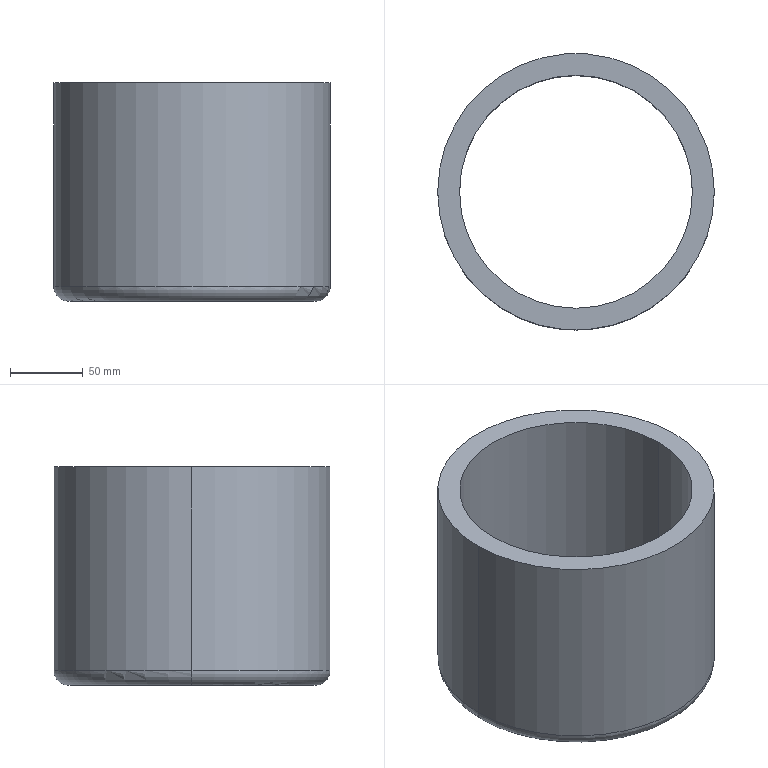Part | SolidWorks | features Extrusion 1, Fillet 1 | 1 solid | 8 faces | box 190 x 190 x 150 mm | volume 1224494 mm3 | cylinder 4 | torus 2 | plane 2 | commonest cylinder face diameters 160 x2 190 x2
STEP:
#1=CARTESIAN_POINT('',(-684.884,-90.,-50.));
#2=VERTEX_POINT('',#1);
#3=CARTESIAN_POINT('',(-514.884,-90.,-50.));
#4=VERTEX_POINT('',#3);
#5=CARTESIAN_POINT('',(-599.884,-90.,-50.));
#6=DIRECTION('',(0.,0.,-1.));
#7=DIRECTION('',(1.,0.,0.));
#8=AXIS2_PLACEMENT_3D('',#5,#6,#7);
#9=CIRCLE('',#8,85.);
#10=EDGE_CURVE('',#2,#4,#9,.T.);
#11=ORIENTED_EDGE('',*,*,#10,.F.);
#12=CARTESIAN_POINT('',(-694.884,-90.,-40.));
#13=VERTEX_POINT('',#12);
#14=CARTESIAN_POINT('',(-684.884,-90.,-40.));
#15=DIRECTION('',(0.,1.,0.));
#16=DIRECTION('',(-1.,0.,0.));
#17=AXIS2_PLACEMENT_3D('',#14,#15,#16);
#18=CIRCLE('',#17,10.);
#19=EDGE_CURVE('',#2,#13,#18,.T.);
#20=ORIENTED_EDGE('',*,*,#19,.T.);
#21=CARTESIAN_POINT('',(-504.884,-90.,-40.));
#22=VERTEX_POINT('',#21);
#23=CARTESIAN_POINT('',(-599.884,-90.,-40.));
#24=DIRECTION('',(0.,0.,1.));
#25=DIRECTION('',(1.,0.,0.));
#26=AXIS2_PLACEMENT_3D('',#23,#24,#25);
#27=CIRCLE('',#26,95.);
#28=EDGE_CURVE('',#22,#13,#27,.T.);
#29=ORIENTED_EDGE('',*,*,#28,.F.);
#30=CARTESIAN_POINT('',(-514.884,-90.,-40.));
#31=DIRECTION('',(0.,-1.,0.));
#32=DIRECTION('',(0.,0.,-1.));
#33=AXIS2_PLACEMENT_3D('',#30,#31,#32);
#34=CIRCLE('',#33,10.);
#35=EDGE_CURVE('',#4,#22,#34,.T.);
#36=ORIENTED_EDGE('',*,*,#35,.F.);
#37=EDGE_LOOP('',(#11,#20,#29,#36));
#38=FACE_OUTER_BOUND('',#37,.T.);
#39=CARTESIAN_POINT('',(-599.884,-90.,-40.));
#40=DIRECTION('',(0.,0.,1.));
#41=DIRECTION('',(1.,0.,0.));
#42=AXIS2_PLACEMENT_3D('',#39,#40,#41);
#43=TOROIDAL_SURFACE('',#42,85.,10.);
#44=ADVANCED_FACE('',(#38),#43,.T.);
#45=CARTESIAN_POINT('',(-679.884,-90.,-50.));
#46=VERTEX_POINT('',#45);
#47=CARTESIAN_POINT('',(-519.884,-90.,-50.));
#48=VERTEX_POINT('',#47);
#49=CARTESIAN_POINT('',(-599.884,-90.,-50.));
#50=DIRECTION('',(0.,0.,1.));
#51=DIRECTION('',(1.,0.,0.));
#52=AXIS2_PLACEMENT_3D('',#49,#50,#51);
#53=CIRCLE('',#52,80.);
#54=EDGE_CURVE('',#46,#48,#53,.T.);
#55=ORIENTED_EDGE('',*,*,#54,.F.);
#56=CARTESIAN_POINT('',(-679.884,-90.,100.));
#57=VERTEX_POINT('',#56);
#58=CARTESIAN_POINT('',(-679.884,-90.,-50.));
#59=DIRECTION('',(0.,0.,1.));
#60=VECTOR('',#59,1000.);
#61=LINE('',#58,#60);
#62=EDGE_CURVE('',#46,#57,#61,.T.);
#63=ORIENTED_EDGE('',*,*,#62,.T.);
#64=CARTESIAN_POINT('',(-519.884,-90.,100.));
#65=VERTEX_POINT('',#64);
#66=CARTESIAN_POINT('',(-599.884,-90.,100.));
#67=DIRECTION('',(0.,0.,1.));
#68=DIRECTION('',(1.,0.,0.));
#69=AXIS2_PLACEMENT_3D('',#66,#67,#68);
#70=CIRCLE('',#69,80.);
#71=EDGE_CURVE('',#57,#65,#70,.T.);
#72=ORIENTED_EDGE('',*,*,#71,.T.);
#73=CARTESIAN_POINT('',(-519.884,-90.,-50.));
#74=DIRECTION('',(0.,0.,1.));
#75=VECTOR('',#74,1000.);
#76=LINE('',#73,#75);
#77=EDGE_CURVE('',#48,#65,#76,.T.);
#78=ORIENTED_EDGE('',*,*,#77,.F.);
#79=EDGE_LOOP('',(#55,#63,#72,#78));
#80=FACE_OUTER_BOUND('',#79,.T.);
#81=CARTESIAN_POINT('',(-599.884,-90.,-50.));
#82=DIRECTION('',(0.,0.,1.));
#83=DIRECTION('',(1.,0.,0.));
#84=AXIS2_PLACEMENT_3D('',#81,#82,#83);
#85=CYLINDRICAL_SURFACE('',#84,80.);
#86=ADVANCED_FACE('',(#80),#85,.F.);
#87=ORIENTED_EDGE('',*,*,#28,.T.);
#88=CARTESIAN_POINT('',(-694.884,-90.,100.));
#89=VERTEX_POINT('',#88);
#90=CARTESIAN_POINT('',(-694.884,-90.,-50.));
#91=DIRECTION('',(0.,0.,1.));
#92=VECTOR('',#91,1000.);
#93=LINE('',#90,#92);
#94=EDGE_CURVE('',#13,#89,#93,.T.);
#95=ORIENTED_EDGE('',*,*,#94,.T.);
#96=CARTESIAN_POINT('',(-504.884,-90.,100.));
#97=VERTEX_POINT('',#96);
#98=CARTESIAN_POINT('',(-599.884,-90.,100.));
#99=DIRECTION('',(0.,0.,1.));
#100=DIRECTION('',(1.,0.,0.));
#101=AXIS2_PLACEMENT_3D('',#98,#99,#100);
#102=CIRCLE('',#101,95.);
#103=EDGE_CURVE('',#97,#89,#102,.T.);
#104=ORIENTED_EDGE('',*,*,#103,.F.);
#105=CARTESIAN_POINT('',(-504.884,-90.,-50.));
#106=DIRECTION('',(0.,0.,1.));
#107=VECTOR('',#106,1000.);
#108=LINE('',#105,#107);
#109=EDGE_CURVE('',#22,#97,#108,.T.);
#110=ORIENTED_EDGE('',*,*,#109,.F.);
#111=EDGE_LOOP('',(#87,#95,#104,#110));
#112=FACE_OUTER_BOUND('',#111,.T.);
#113=CARTESIAN_POINT('',(-599.884,-90.,-50.));
#114=DIRECTION('',(0.,0.,1.));
#115=DIRECTION('',(1.,0.,0.));
#116=AXIS2_PLACEMENT_3D('',#113,#114,#115);
#117=CYLINDRICAL_SURFACE('',#116,95.);
#118=ADVANCED_FACE('',(#112),#117,.T.);
#119=ORIENTED_EDGE('',*,*,#94,.F.);
#120=CARTESIAN_POINT('',(-599.884,-90.,-40.));
#121=DIRECTION('',(0.,0.,1.));
#122=DIRECTION('',(1.,0.,0.));
#123=AXIS2_PLACEMENT_3D('',#120,#121,#122);
#124=CIRCLE('',#123,95.);
#125=EDGE_CURVE('',#13,#22,#124,.T.);
#126=ORIENTED_EDGE('',*,*,#125,.T.);
#127=ORIENTED_EDGE('',*,*,#109,.T.);
#128=CARTESIAN_POINT('',(-599.884,-90.,100.));
#129=DIRECTION('',(0.,0.,1.));
#130=DIRECTION('',(1.,0.,0.));
#131=AXIS2_PLACEMENT_3D('',#128,#129,#130);
#132=CIRCLE('',#131,95.);
#133=EDGE_CURVE('',#89,#97,#132,.T.);
#134=ORIENTED_EDGE('',*,*,#133,.F.);
#135=EDGE_LOOP('',(#119,#126,#127,#134));
#136=FACE_OUTER_BOUND('',#135,.T.);
#137=CARTESIAN_POINT('',(-599.884,-90.,-50.));
#138=DIRECTION('',(0.,0.,1.));
#139=DIRECTION('',(1.,0.,0.));
#140=AXIS2_PLACEMENT_3D('',#137,#138,#139);
#141=CYLINDRICAL_SURFACE('',#140,95.);
#142=ADVANCED_FACE('',(#136),#141,.T.);
#143=CARTESIAN_POINT('',(-599.884,-90.,-50.));
#144=DIRECTION('',(0.,0.,-1.));
#145=DIRECTION('',(1.,0.,0.));
#146=AXIS2_PLACEMENT_3D('',#143,#144,#145);
#147=CIRCLE('',#146,85.);
#148=EDGE_CURVE('',#4,#2,#147,.T.);
#149=ORIENTED_EDGE('',*,*,#148,.T.);
#150=ORIENTED_EDGE('',*,*,#10,.T.);
#151=EDGE_LOOP('',(#149,#150));
#152=FACE_OUTER_BOUND('',#151,.T.);
#153=CARTESIAN_POINT('',(-599.884,-90.,-50.));
#154=DIRECTION('',(0.,0.,1.));
#155=DIRECTION('',(1.,0.,0.));
#156=AXIS2_PLACEMENT_3D('',#153,#154,#155);
#157=CIRCLE('',#156,80.);
#158=EDGE_CURVE('',#48,#46,#157,.T.);
#159=ORIENTED_EDGE('',*,*,#158,.T.);
#160=ORIENTED_EDGE('',*,*,#54,.T.);
#161=EDGE_LOOP('',(#159,#160));
#162=FACE_BOUND('',#161,.T.);
#163=CARTESIAN_POINT('',(-599.884,-90.,-50.));
#164=DIRECTION('',(0.,0.,1.));
#165=DIRECTION('',(1.,0.,0.));
#166=AXIS2_PLACEMENT_3D('',#163,#164,#165);
#167=PLANE('',#166);
#168=ADVANCED_FACE('',(#152,#162),#167,.F.);
#169=ORIENTED_EDGE('',*,*,#62,.F.);
#170=ORIENTED_EDGE('',*,*,#158,.F.);
#171=ORIENTED_EDGE('',*,*,#77,.T.);
#172=CARTESIAN_POINT('',(-599.884,-90.,100.));
#173=DIRECTION('',(0.,0.,1.));
#174=DIRECTION('',(1.,0.,0.));
#175=AXIS2_PLACEMENT_3D('',#172,#173,#174);
#176=CIRCLE('',#175,80.);
#177=EDGE_CURVE('',#65,#57,#176,.T.);
#178=ORIENTED_EDGE('',*,*,#177,.T.);
#179=EDGE_LOOP('',(#169,#170,#171,#178));
#180=FACE_OUTER_BOUND('',#179,.T.);
#181=CARTESIAN_POINT('',(-599.884,-90.,-50.));
#182=DIRECTION('',(0.,0.,1.));
#183=DIRECTION('',(1.,0.,0.));
#184=AXIS2_PLACEMENT_3D('',#181,#182,#183);
#185=CYLINDRICAL_SURFACE('',#184,80.);
#186=ADVANCED_FACE('',(#180),#185,.F.);
#187=ORIENTED_EDGE('',*,*,#103,.T.);
#188=ORIENTED_EDGE('',*,*,#133,.T.);
#189=EDGE_LOOP('',(#187,#188));
#190=FACE_OUTER_BOUND('',#189,.T.);
#191=ORIENTED_EDGE('',*,*,#177,.F.);
#192=ORIENTED_EDGE('',*,*,#71,.F.);
#193=EDGE_LOOP('',(#191,#192));
#194=FACE_BOUND('',#193,.T.);
#195=CARTESIAN_POINT('',(-599.884,-90.,100.));
#196=DIRECTION('',(0.,0.,1.));
#197=DIRECTION('',(1.,0.,0.));
#198=AXIS2_PLACEMENT_3D('',#195,#196,#197);
#199=PLANE('',#198);
#200=ADVANCED_FACE('',(#190,#194),#199,.T.);
#201=ORIENTED_EDGE('',*,*,#19,.F.);
#202=ORIENTED_EDGE('',*,*,#148,.F.);
#203=ORIENTED_EDGE('',*,*,#35,.T.);
#204=ORIENTED_EDGE('',*,*,#125,.F.);
#205=EDGE_LOOP('',(#201,#202,#203,#204));
#206=FACE_OUTER_BOUND('',#205,.T.);
#207=CARTESIAN_POINT('',(-599.884,-90.,-40.));
#208=DIRECTION('',(0.,0.,1.));
#209=DIRECTION('',(1.,0.,0.));
#210=AXIS2_PLACEMENT_3D('',#207,#208,#209);
#211=TOROIDAL_SURFACE('',#210,85.,10.);
#212=ADVANCED_FACE('',(#206),#211,.T.);
#213=CLOSED_SHELL('',(#44,#86,#118,#142,#168,#186,#200,#212));
#214=MANIFOLD_SOLID_BREP('',#213);
#215=CARTESIAN_POINT('',(0.,0.,0.));
#216=DIRECTION('',(0.,0.,1.));
#217=DIRECTION('',(1.,0.,0.));
#218=AXIS2_PLACEMENT_3D('',#215,#216,#217);
#219=(LENGTH_UNIT()NAMED_UNIT(*)SI_UNIT(.MILLI.,.METRE.));
#220=UNCERTAINTY_MEASURE_WITH_UNIT(LENGTH_MEASURE(0.00001),#219,'','');
#221=(NAMED_UNIT(*)PLANE_ANGLE_UNIT()SI_UNIT($,.RADIAN.));
#222=(NAMED_UNIT(*)SI_UNIT($,.STERADIAN.)SOLID_ANGLE_UNIT());
#223=(GEOMETRIC_REPRESENTATION_CONTEXT(3)GLOBAL_UNCERTAINTY_ASSIGNED_CONTEXT((#220))GLOBAL_UNIT_ASSIGNED_CONTEXT((#219,#221,#222))REPRESENTATION_CONTEXT('',''));
#224=ADVANCED_BREP_SHAPE_REPRESENTATION('',(#214,#218),#223);